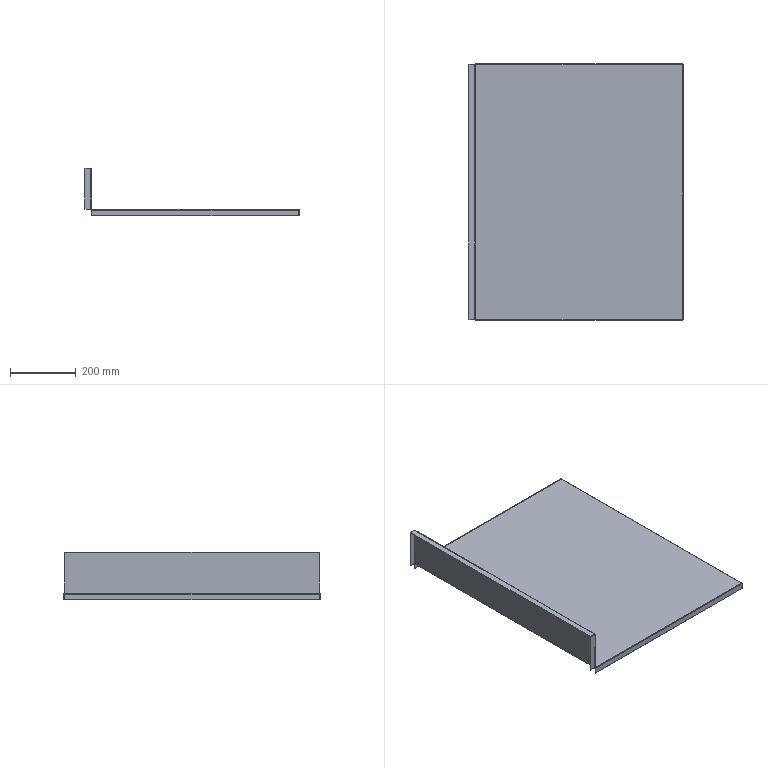Part | STEP file | X77-03022 | 1 solid | 66 faces | box 650 x 778 x 145 mm | volume 963371 mm3 | plane 44 | cylinder 14 | spline 8 | commonest cylinder face diameters 1.473 x7 4.473 x7